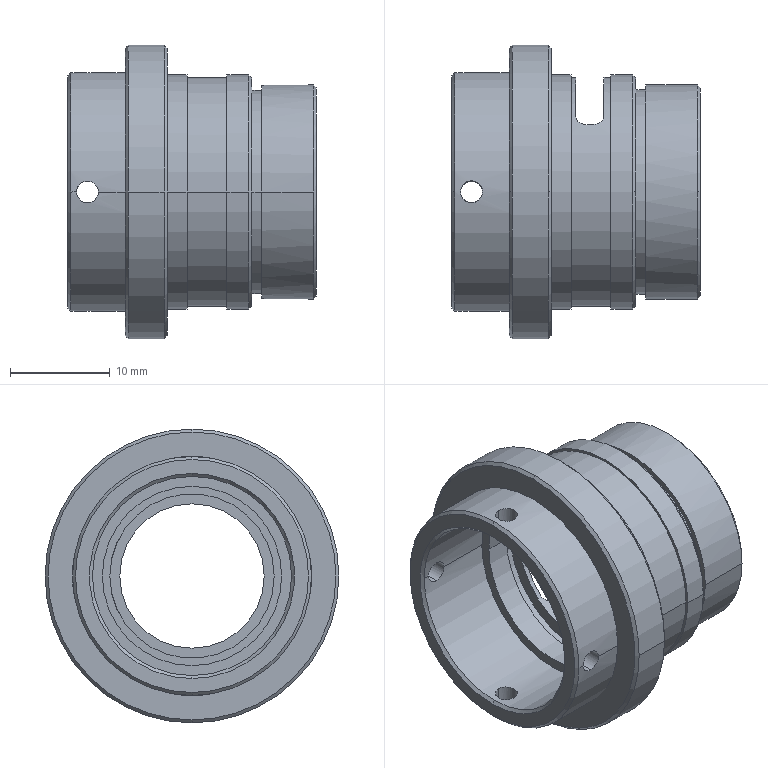Part | STEP file | aperture tube.stp.STEP-219.STEP | 1 solid | 66 faces | box 25 x 29.5 x 29.5 mm | volume 5283 mm3 | cylinder 36 | plane 16 | cone 14 | commonest cylinder face diameters 2.2 x8 2 x4 23.5 x4 14.5 x2 16.5 x2 18 x2